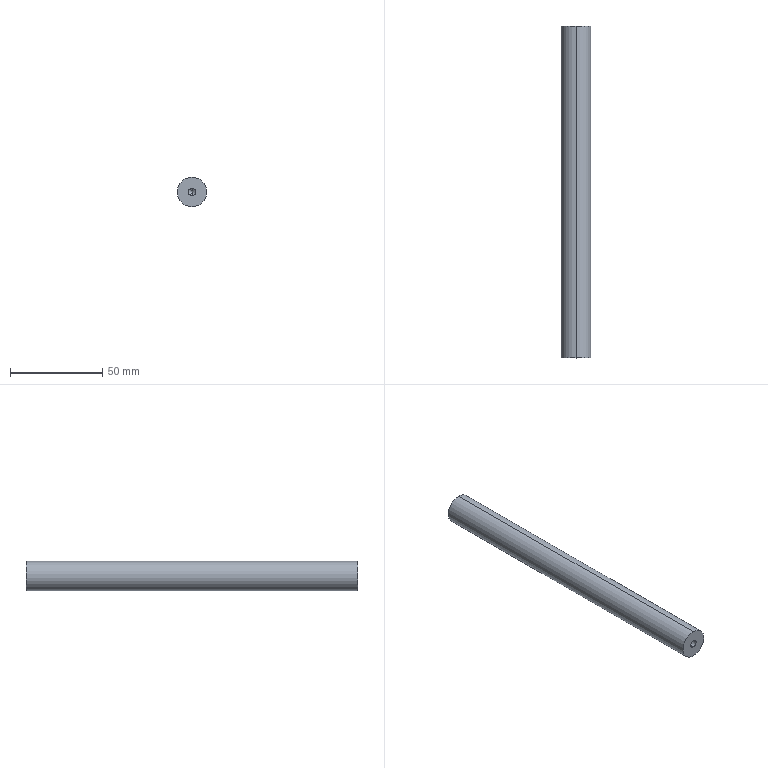Part | STEP file | PSFJW16-180-M5-N5 | 1 solid | 12 faces | box 16 x 180 x 16 mm | volume 35836 mm3 | cylinder 6 | cone 4 | plane 2 | commonest cylinder face diameters 4.2 x4 16 x2
STEP:
#1=CARTESIAN_POINT('',(0.,0.,0.));
#2=DIRECTION('',(0.,0.,1.));
#3=DIRECTION('',(1.,0.,0.));
#4=AXIS2_PLACEMENT_3D('',#1,#2,#3);
#5=CARTESIAN_POINT('',(0.,12.4,-2.1));
#6=VERTEX_POINT('',#5);
#7=CARTESIAN_POINT('',(0.,0.,-2.1));
#8=VERTEX_POINT('',#7);
#9=CARTESIAN_POINT('',(0.,0.,-2.1));
#10=DIRECTION('',(0.,-1.,0.));
#11=VECTOR('',#10,1.);
#12=LINE('',#9,#11);
#13=CARTESIAN_POINT('',(0.,0.,0.));
#14=DIRECTION('',(0.,-1.,0.));
#15=DIRECTION('',(0.,0.,-1.));
#16=AXIS2_PLACEMENT_3D('',#13,#14,#15);
#17=CYLINDRICAL_SURFACE('',#16,2.1);
#18=CARTESIAN_POINT('',(6.283,0.));
#19=DIRECTION('',(0.,1.));
#20=VECTOR('',#19,1.);
#21=LINE('',#18,#20);
#22=(GEOMETRIC_REPRESENTATION_CONTEXT(2)PARAMETRIC_REPRESENTATION_CONTEXT()REPRESENTATION_CONTEXT('',''));
#23=DEFINITIONAL_REPRESENTATION('',(#21),#22);
#24=PCURVE('',#17,#23);
#25=CARTESIAN_POINT('',(0.,0.,0.));
#26=DIRECTION('',(0.,-1.,0.));
#27=DIRECTION('',(0.,0.,-1.));
#28=AXIS2_PLACEMENT_3D('',#25,#26,#27);
#29=CYLINDRICAL_SURFACE('',#28,2.1);
#30=CARTESIAN_POINT('',(0.,0.));
#31=DIRECTION('',(0.,1.));
#32=VECTOR('',#31,1.);
#33=LINE('',#30,#32);
#34=(GEOMETRIC_REPRESENTATION_CONTEXT(2)PARAMETRIC_REPRESENTATION_CONTEXT()REPRESENTATION_CONTEXT('',''));
#35=DEFINITIONAL_REPRESENTATION('',(#33),#34);
#36=PCURVE('',#29,#35);
#37=SURFACE_CURVE('',#12,(#24,#36),.PCURVE_S1.);
#38=EDGE_CURVE('',#6,#8,#37,.T.);
#39=ORIENTED_EDGE('',*,*,#38,.T.);
#40=CARTESIAN_POINT('',(0.,0.,2.1));
#41=VERTEX_POINT('',#40);
#42=CARTESIAN_POINT('',(0.,0.,0.));
#43=DIRECTION('',(0.,-1.,0.));
#44=DIRECTION('',(0.,0.,-1.));
#45=AXIS2_PLACEMENT_3D('',#42,#43,#44);
#46=CIRCLE('',#45,2.1);
#47=CARTESIAN_POINT('',(0.,0.));
#48=DIRECTION('',(1.,0.));
#49=VECTOR('',#48,1.);
#50=LINE('',#47,#49);
#51=(GEOMETRIC_REPRESENTATION_CONTEXT(2)PARAMETRIC_REPRESENTATION_CONTEXT()REPRESENTATION_CONTEXT('',''));
#52=DEFINITIONAL_REPRESENTATION('',(#50),#51);
#53=PCURVE('',#17,#52);
#54=CARTESIAN_POINT('',(0.,0.,0.));
#55=DIRECTION('',(0.,1.,0.));
#56=DIRECTION('',(0.,0.,1.));
#57=AXIS2_PLACEMENT_3D('',#54,#55,#56);
#58=PLANE('',#57);
#59=CARTESIAN_POINT('',(-2.1,0.));
#60=CARTESIAN_POINT('',(-2.1,3.637));
#61=CARTESIAN_POINT('',(1.05,1.819));
#62=CARTESIAN_POINT('',(4.2,0.));
#63=CARTESIAN_POINT('',(1.05,-1.819));
#64=CARTESIAN_POINT('',(-2.1,-3.637));
#65=CARTESIAN_POINT('',(-2.1,0.));
#66=(BOUNDED_CURVE()B_SPLINE_CURVE(2,(#59,#60,#61,#62,#63,#64,#65),.UNSPECIFIED.,.T.,.F.)B_SPLINE_CURVE_WITH_KNOTS((1,2,2,2,2,1),(-2.094,0.,2.094,4.189,6.283,8.378),.UNSPECIFIED.)CURVE()GEOMETRIC_REPRESENTATION_ITEM()RATIONAL_B_SPLINE_CURVE((1.,0.5,1.,0.5,1.,0.5,1.))REPRESENTATION_ITEM(''));
#67=(GEOMETRIC_REPRESENTATION_CONTEXT(2)PARAMETRIC_REPRESENTATION_CONTEXT()REPRESENTATION_CONTEXT('',''));
#68=DEFINITIONAL_REPRESENTATION('',(#66),#67);
#69=PCURVE('',#58,#68);
#70=SURFACE_CURVE('',#46,(#53,#69),.PCURVE_S1.);
#71=EDGE_CURVE('',#41,#8,#70,.T.);
#72=ORIENTED_EDGE('',*,*,#71,.F.);
#73=CARTESIAN_POINT('',(0.,12.4,2.1));
#74=VERTEX_POINT('',#73);
#75=CARTESIAN_POINT('',(0.,0.,2.1));
#76=DIRECTION('',(0.,-1.,0.));
#77=VECTOR('',#76,1.);
#78=LINE('',#75,#77);
#79=CARTESIAN_POINT('',(3.142,0.));
#80=DIRECTION('',(0.,1.));
#81=VECTOR('',#80,1.);
#82=LINE('',#79,#81);
#83=(GEOMETRIC_REPRESENTATION_CONTEXT(2)PARAMETRIC_REPRESENTATION_CONTEXT()REPRESENTATION_CONTEXT('',''));
#84=DEFINITIONAL_REPRESENTATION('',(#82),#83);
#85=PCURVE('',#17,#84);
#86=CARTESIAN_POINT('',(3.142,0.));
#87=DIRECTION('',(0.,1.));
#88=VECTOR('',#87,1.);
#89=LINE('',#86,#88);
#90=(GEOMETRIC_REPRESENTATION_CONTEXT(2)PARAMETRIC_REPRESENTATION_CONTEXT()REPRESENTATION_CONTEXT('',''));
#91=DEFINITIONAL_REPRESENTATION('',(#89),#90);
#92=PCURVE('',#29,#91);
#93=SURFACE_CURVE('',#78,(#85,#92),.PCURVE_S1.);
#94=EDGE_CURVE('',#74,#41,#93,.T.);
#95=ORIENTED_EDGE('',*,*,#94,.F.);
#96=CARTESIAN_POINT('',(0.,12.4,0.));
#97=DIRECTION('',(0.,-1.,0.));
#98=DIRECTION('',(0.,0.,-1.));
#99=AXIS2_PLACEMENT_3D('',#96,#97,#98);
#100=CIRCLE('',#99,2.1);
#101=CARTESIAN_POINT('',(0.,-12.4));
#102=DIRECTION('',(1.,0.));
#103=VECTOR('',#102,1.);
#104=LINE('',#101,#103);
#105=(GEOMETRIC_REPRESENTATION_CONTEXT(2)PARAMETRIC_REPRESENTATION_CONTEXT()REPRESENTATION_CONTEXT('',''));
#106=DEFINITIONAL_REPRESENTATION('',(#104),#105);
#107=PCURVE('',#17,#106);
#108=CARTESIAN_POINT('',(0.,12.4,0.));
#109=DIRECTION('',(0.,-1.,0.));
#110=DIRECTION('',(0.,0.,-1.));
#111=AXIS2_PLACEMENT_3D('',#108,#109,#110);
#112=CONICAL_SURFACE('',#111,2.1,1.03);
#113=CARTESIAN_POINT('',(0.,0.));
#114=DIRECTION('',(1.,0.));
#115=VECTOR('',#114,1.);
#116=LINE('',#113,#115);
#117=(GEOMETRIC_REPRESENTATION_CONTEXT(2)PARAMETRIC_REPRESENTATION_CONTEXT()REPRESENTATION_CONTEXT('',''));
#118=DEFINITIONAL_REPRESENTATION('',(#116),#117);
#119=PCURVE('',#112,#118);
#120=SURFACE_CURVE('',#100,(#107,#119),.PCURVE_S1.);
#121=EDGE_CURVE('',#74,#6,#120,.T.);
#122=ORIENTED_EDGE('',*,*,#121,.T.);
#123=EDGE_LOOP('',(#39,#72,#95,#122));
#124=FACE_BOUND('',#123,.F.);
#125=ADVANCED_FACE('',(#124),#17,.F.);
#126=ORIENTED_EDGE('',*,*,#121,.F.);
#127=CARTESIAN_POINT('',(0.,13.662,0.));
#128=VERTEX_POINT('',#127);
#129=CARTESIAN_POINT('',(0.,12.4,2.1));
#130=DIRECTION('',(0.,-0.515,0.8572));
#131=VECTOR('',#130,1.);
#132=LINE('',#129,#131);
#133=CARTESIAN_POINT('',(3.142,0.));
#134=DIRECTION('',(0.,1.));
#135=VECTOR('',#134,1.);
#136=LINE('',#133,#135);
#137=(GEOMETRIC_REPRESENTATION_CONTEXT(2)PARAMETRIC_REPRESENTATION_CONTEXT()REPRESENTATION_CONTEXT('',''));
#138=DEFINITIONAL_REPRESENTATION('',(#136),#137);
#139=PCURVE('',#112,#138);
#140=CARTESIAN_POINT('',(0.,12.4,0.));
#141=DIRECTION('',(0.,-1.,0.));
#142=DIRECTION('',(0.,0.,-1.));
#143=AXIS2_PLACEMENT_3D('',#140,#141,#142);
#144=CONICAL_SURFACE('',#143,2.1,1.03);
#145=CARTESIAN_POINT('',(3.142,0.));
#146=DIRECTION('',(0.,1.));
#147=VECTOR('',#146,1.);
#148=LINE('',#145,#147);
#149=(GEOMETRIC_REPRESENTATION_CONTEXT(2)PARAMETRIC_REPRESENTATION_CONTEXT()REPRESENTATION_CONTEXT('',''));
#150=DEFINITIONAL_REPRESENTATION('',(#148),#149);
#151=PCURVE('',#144,#150);
#152=SURFACE_CURVE('',#132,(#139,#151),.PCURVE_S1.);
#153=EDGE_CURVE('',#128,#74,#152,.T.);
#154=ORIENTED_EDGE('',*,*,#153,.F.);
#155=CARTESIAN_POINT('',(0.,12.4,-2.1));
#156=DIRECTION('',(0.,-0.515,-0.8572));
#157=VECTOR('',#156,1.);
#158=LINE('',#155,#157);
#159=CARTESIAN_POINT('',(6.283,0.));
#160=DIRECTION('',(0.,1.));
#161=VECTOR('',#160,1.);
#162=LINE('',#159,#161);
#163=(GEOMETRIC_REPRESENTATION_CONTEXT(2)PARAMETRIC_REPRESENTATION_CONTEXT()REPRESENTATION_CONTEXT('',''));
#164=DEFINITIONAL_REPRESENTATION('',(#162),#163);
#165=PCURVE('',#112,#164);
#166=CARTESIAN_POINT('',(0.,0.));
#167=DIRECTION('',(0.,1.));
#168=VECTOR('',#167,1.);
#169=LINE('',#166,#168);
#170=(GEOMETRIC_REPRESENTATION_CONTEXT(2)PARAMETRIC_REPRESENTATION_CONTEXT()REPRESENTATION_CONTEXT('',''));
#171=DEFINITIONAL_REPRESENTATION('',(#169),#170);
#172=PCURVE('',#144,#171);
#173=SURFACE_CURVE('',#158,(#165,#172),.PCURVE_S1.);
#174=EDGE_CURVE('',#128,#6,#173,.T.);
#175=ORIENTED_EDGE('',*,*,#174,.T.);
#176=EDGE_LOOP('',(#126,#154,#175));
#177=FACE_BOUND('',#176,.F.);
#178=ADVANCED_FACE('',(#177),#112,.F.);
#179=CARTESIAN_POINT('',(0.,167.6,2.1));
#180=VERTEX_POINT('',#179);
#181=CARTESIAN_POINT('',(0.,180.,2.1));
#182=VERTEX_POINT('',#181);
#183=CARTESIAN_POINT('',(0.,180.,2.1));
#184=DIRECTION('',(0.,1.,0.));
#185=VECTOR('',#184,1.);
#186=LINE('',#183,#185);
#187=CARTESIAN_POINT('',(0.,180.,0.));
#188=DIRECTION('',(0.,1.,0.));
#189=DIRECTION('',(0.,0.,1.));
#190=AXIS2_PLACEMENT_3D('',#187,#188,#189);
#191=CYLINDRICAL_SURFACE('',#190,2.1);
#192=CARTESIAN_POINT('',(6.283,0.));
#193=DIRECTION('',(0.,1.));
#194=VECTOR('',#193,1.);
#195=LINE('',#192,#194);
#196=(GEOMETRIC_REPRESENTATION_CONTEXT(2)PARAMETRIC_REPRESENTATION_CONTEXT()REPRESENTATION_CONTEXT('',''));
#197=DEFINITIONAL_REPRESENTATION('',(#195),#196);
#198=PCURVE('',#191,#197);
#199=CARTESIAN_POINT('',(0.,180.,0.));
#200=DIRECTION('',(0.,1.,0.));
#201=DIRECTION('',(0.,0.,1.));
#202=AXIS2_PLACEMENT_3D('',#199,#200,#201);
#203=CYLINDRICAL_SURFACE('',#202,2.1);
#204=CARTESIAN_POINT('',(0.,0.));
#205=DIRECTION('',(0.,1.));
#206=VECTOR('',#205,1.);
#207=LINE('',#204,#206);
#208=(GEOMETRIC_REPRESENTATION_CONTEXT(2)PARAMETRIC_REPRESENTATION_CONTEXT()REPRESENTATION_CONTEXT('',''));
#209=DEFINITIONAL_REPRESENTATION('',(#207),#208);
#210=PCURVE('',#203,#209);
#211=SURFACE_CURVE('',#186,(#198,#210),.PCURVE_S1.);
#212=EDGE_CURVE('',#180,#182,#211,.T.);
#213=ORIENTED_EDGE('',*,*,#212,.T.);
#214=CARTESIAN_POINT('',(0.,180.,-2.1));
#215=VERTEX_POINT('',#214);
#216=CARTESIAN_POINT('',(0.,180.,0.));
#217=DIRECTION('',(0.,1.,0.));
#218=DIRECTION('',(0.,0.,1.));
#219=AXIS2_PLACEMENT_3D('',#216,#217,#218);
#220=CIRCLE('',#219,2.1);
#221=CARTESIAN_POINT('',(0.,0.));
#222=DIRECTION('',(1.,0.));
#223=VECTOR('',#222,1.);
#224=LINE('',#221,#223);
#225=(GEOMETRIC_REPRESENTATION_CONTEXT(2)PARAMETRIC_REPRESENTATION_CONTEXT()REPRESENTATION_CONTEXT('',''));
#226=DEFINITIONAL_REPRESENTATION('',(#224),#225);
#227=PCURVE('',#191,#226);
#228=CARTESIAN_POINT('',(0.,180.,0.));
#229=DIRECTION('',(0.,1.,0.));
#230=DIRECTION('',(0.,0.,1.));
#231=AXIS2_PLACEMENT_3D('',#228,#229,#230);
#232=PLANE('',#231);
#233=CARTESIAN_POINT('',(0.,0.));
#234=DIRECTION('',(1.,0.));
#235=AXIS2_PLACEMENT_2D('',#233,#234);
#236=CIRCLE('',#235,2.1);
#237=(GEOMETRIC_REPRESENTATION_CONTEXT(2)PARAMETRIC_REPRESENTATION_CONTEXT()REPRESENTATION_CONTEXT('',''));
#238=DEFINITIONAL_REPRESENTATION('',(#236),#237);
#239=PCURVE('',#232,#238);
#240=SURFACE_CURVE('',#220,(#227,#239),.PCURVE_S1.);
#241=EDGE_CURVE('',#215,#182,#240,.T.);
#242=ORIENTED_EDGE('',*,*,#241,.F.);
#243=CARTESIAN_POINT('',(0.,167.6,-2.1));
#244=VERTEX_POINT('',#243);
#245=CARTESIAN_POINT('',(0.,180.,-2.1));
#246=DIRECTION('',(0.,1.,0.));
#247=VECTOR('',#246,1.);
#248=LINE('',#245,#247);
#249=CARTESIAN_POINT('',(3.142,0.));
#250=DIRECTION('',(0.,1.));
#251=VECTOR('',#250,1.);
#252=LINE('',#249,#251);
#253=(GEOMETRIC_REPRESENTATION_CONTEXT(2)PARAMETRIC_REPRESENTATION_CONTEXT()REPRESENTATION_CONTEXT('',''));
#254=DEFINITIONAL_REPRESENTATION('',(#252),#253);
#255=PCURVE('',#191,#254);
#256=CARTESIAN_POINT('',(3.142,0.));
#257=DIRECTION('',(0.,1.));
#258=VECTOR('',#257,1.);
#259=LINE('',#256,#258);
#260=(GEOMETRIC_REPRESENTATION_CONTEXT(2)PARAMETRIC_REPRESENTATION_CONTEXT()REPRESENTATION_CONTEXT('',''));
#261=DEFINITIONAL_REPRESENTATION('',(#259),#260);
#262=PCURVE('',#203,#261);
#263=SURFACE_CURVE('',#248,(#255,#262),.PCURVE_S1.);
#264=EDGE_CURVE('',#244,#215,#263,.T.);
#265=ORIENTED_EDGE('',*,*,#264,.F.);
#266=CARTESIAN_POINT('',(0.,167.6,0.));
#267=DIRECTION('',(0.,1.,0.));
#268=DIRECTION('',(0.,0.,1.));
#269=AXIS2_PLACEMENT_3D('',#266,#267,#268);
#270=CIRCLE('',#269,2.1);
#271=CARTESIAN_POINT('',(0.,-12.4));
#272=DIRECTION('',(1.,0.));
#273=VECTOR('',#272,1.);
#274=LINE('',#271,#273);
#275=(GEOMETRIC_REPRESENTATION_CONTEXT(2)PARAMETRIC_REPRESENTATION_CONTEXT()REPRESENTATION_CONTEXT('',''));
#276=DEFINITIONAL_REPRESENTATION('',(#274),#275);
#277=PCURVE('',#191,#276);
#278=CARTESIAN_POINT('',(0.,167.6,0.));
#279=DIRECTION('',(0.,1.,0.));
#280=DIRECTION('',(0.,0.,1.));
#281=AXIS2_PLACEMENT_3D('',#278,#279,#280);
#282=CONICAL_SURFACE('',#281,2.1,1.03);
#283=CARTESIAN_POINT('',(0.,0.));
#284=DIRECTION('',(1.,0.));
#285=VECTOR('',#284,1.);
#286=LINE('',#283,#285);
#287=(GEOMETRIC_REPRESENTATION_CONTEXT(2)PARAMETRIC_REPRESENTATION_CONTEXT()REPRESENTATION_CONTEXT('',''));
#288=DEFINITIONAL_REPRESENTATION('',(#286),#287);
#289=PCURVE('',#282,#288);
#290=SURFACE_CURVE('',#270,(#277,#289),.PCURVE_S1.);
#291=EDGE_CURVE('',#244,#180,#290,.T.);
#292=ORIENTED_EDGE('',*,*,#291,.T.);
#293=EDGE_LOOP('',(#213,#242,#265,#292));
#294=FACE_BOUND('',#293,.F.);
#295=ADVANCED_FACE('',(#294),#191,.F.);
#296=ORIENTED_EDGE('',*,*,#291,.F.);
#297=CARTESIAN_POINT('',(0.,166.338,0.));
#298=VERTEX_POINT('',#297);
#299=CARTESIAN_POINT('',(0.,167.6,-2.1));
#300=DIRECTION('',(0.,0.515,-0.8572));
#301=VECTOR('',#300,1.);
#302=LINE('',#299,#301);
#303=CARTESIAN_POINT('',(3.142,0.));
#304=DIRECTION('',(0.,1.));
#305=VECTOR('',#304,1.);
#306=LINE('',#303,#305);
#307=(GEOMETRIC_REPRESENTATION_CONTEXT(2)PARAMETRIC_REPRESENTATION_CONTEXT()REPRESENTATION_CONTEXT('',''));
#308=DEFINITIONAL_REPRESENTATION('',(#306),#307);
#309=PCURVE('',#282,#308);
#310=CARTESIAN_POINT('',(0.,167.6,0.));
#311=DIRECTION('',(0.,1.,0.));
#312=DIRECTION('',(0.,0.,1.));
#313=AXIS2_PLACEMENT_3D('',#310,#311,#312);
#314=CONICAL_SURFACE('',#313,2.1,1.03);
#315=CARTESIAN_POINT('',(3.142,0.));
#316=DIRECTION('',(0.,1.));
#317=VECTOR('',#316,1.);
#318=LINE('',#315,#317);
#319=(GEOMETRIC_REPRESENTATION_CONTEXT(2)PARAMETRIC_REPRESENTATION_CONTEXT()REPRESENTATION_CONTEXT('',''));
#320=DEFINITIONAL_REPRESENTATION('',(#318),#319);
#321=PCURVE('',#314,#320);
#322=SURFACE_CURVE('',#302,(#309,#321),.PCURVE_S1.);
#323=EDGE_CURVE('',#298,#244,#322,.T.);
#324=ORIENTED_EDGE('',*,*,#323,.F.);
#325=CARTESIAN_POINT('',(0.,167.6,2.1));
#326=DIRECTION('',(0.,0.515,0.8572));
#327=VECTOR('',#326,1.);
#328=LINE('',#325,#327);
#329=CARTESIAN_POINT('',(6.283,0.));
#330=DIRECTION('',(0.,1.));
#331=VECTOR('',#330,1.);
#332=LINE('',#329,#331);
#333=(GEOMETRIC_REPRESENTATION_CONTEXT(2)PARAMETRIC_REPRESENTATION_CONTEXT()REPRESENTATION_CONTEXT('',''));
#334=DEFINITIONAL_REPRESENTATION('',(#332),#333);
#335=PCURVE('',#282,#334);
#336=CARTESIAN_POINT('',(0.,0.));
#337=DIRECTION('',(0.,1.));
#338=VECTOR('',#337,1.);
#339=LINE('',#336,#338);
#340=(GEOMETRIC_REPRESENTATION_CONTEXT(2)PARAMETRIC_REPRESENTATION_CONTEXT()REPRESENTATION_CONTEXT('',''));
#341=DEFINITIONAL_REPRESENTATION('',(#339),#340);
#342=PCURVE('',#314,#341);
#343=SURFACE_CURVE('',#328,(#335,#342),.PCURVE_S1.);
#344=EDGE_CURVE('',#298,#180,#343,.T.);
#345=ORIENTED_EDGE('',*,*,#344,.T.);
#346=EDGE_LOOP('',(#296,#324,#345));
#347=FACE_BOUND('',#346,.F.);
#348=ADVANCED_FACE('',(#347),#282,.F.);
#349=CARTESIAN_POINT('',(0.,180.,8.));
#350=VERTEX_POINT('',#349);
#351=CARTESIAN_POINT('',(0.,180.,-8.));
#352=VERTEX_POINT('',#351);
#353=CARTESIAN_POINT('',(0.,180.,0.));
#354=DIRECTION('',(0.,1.,0.));
#355=DIRECTION('',(0.,0.,1.));
#356=AXIS2_PLACEMENT_3D('',#353,#354,#355);
#357=CIRCLE('',#356,8.);
#358=CARTESIAN_POINT('',(0.,180.,0.));
#359=DIRECTION('',(0.,-1.,0.));
#360=DIRECTION('',(0.,0.,-1.));
#361=AXIS2_PLACEMENT_3D('',#358,#359,#360);
#362=CYLINDRICAL_SURFACE('',#361,8.);
#363=CARTESIAN_POINT('',(3.142,0.));
#364=DIRECTION('',(-1.,0.));
#365=VECTOR('',#364,1.);
#366=LINE('',#363,#365);
#367=(GEOMETRIC_REPRESENTATION_CONTEXT(2)PARAMETRIC_REPRESENTATION_CONTEXT()REPRESENTATION_CONTEXT('',''));
#368=DEFINITIONAL_REPRESENTATION('',(#366),#367);
#369=PCURVE('',#362,#368);
#370=CARTESIAN_POINT('',(0.,0.));
#371=DIRECTION('',(1.,0.));
#372=AXIS2_PLACEMENT_2D('',#370,#371);
#373=CIRCLE('',#372,8.);
#374=(GEOMETRIC_REPRESENTATION_CONTEXT(2)PARAMETRIC_REPRESENTATION_CONTEXT()REPRESENTATION_CONTEXT('',''));
#375=DEFINITIONAL_REPRESENTATION('',(#373),#374);
#376=PCURVE('',#232,#375);
#377=SURFACE_CURVE('',#357,(#369,#376),.PCURVE_S1.);
#378=EDGE_CURVE('',#350,#352,#377,.T.);
#379=ORIENTED_EDGE('',*,*,#378,.F.);
#380=CARTESIAN_POINT('',(0.,0.,8.));
#381=VERTEX_POINT('',#380);
#382=CARTESIAN_POINT('',(0.,180.,8.));
#383=DIRECTION('',(0.,-1.,0.));
#384=VECTOR('',#383,1.);
#385=LINE('',#382,#384);
#386=CARTESIAN_POINT('',(3.142,0.));
#387=DIRECTION('',(0.,1.));
#388=VECTOR('',#387,1.);
#389=LINE('',#386,#388);
#390=(GEOMETRIC_REPRESENTATION_CONTEXT(2)PARAMETRIC_REPRESENTATION_CONTEXT()REPRESENTATION_CONTEXT('',''));
#391=DEFINITIONAL_REPRESENTATION('',(#389),#390);
#392=PCURVE('',#362,#391);
#393=CARTESIAN_POINT('',(0.,180.,0.));
#394=DIRECTION('',(0.,-1.,0.));
#395=DIRECTION('',(0.,0.,-1.));
#396=AXIS2_PLACEMENT_3D('',#393,#394,#395);
#397=CYLINDRICAL_SURFACE('',#396,8.);
#398=CARTESIAN_POINT('',(3.142,0.));
#399=DIRECTION('',(0.,1.));
#400=VECTOR('',#399,1.);
#401=LINE('',#398,#400);
#402=(GEOMETRIC_REPRESENTATION_CONTEXT(2)PARAMETRIC_REPRESENTATION_CONTEXT()REPRESENTATION_CONTEXT('',''));
#403=DEFINITIONAL_REPRESENTATION('',(#401),#402);
#404=PCURVE('',#397,#403);
#405=SURFACE_CURVE('',#385,(#392,#404),.PCURVE_S1.);
#406=EDGE_CURVE('',#350,#381,#405,.T.);
#407=ORIENTED_EDGE('',*,*,#406,.T.);
#408=CARTESIAN_POINT('',(0.,0.,-8.));
#409=VERTEX_POINT('',#408);
#410=CARTESIAN_POINT('',(0.,0.,0.));
#411=DIRECTION('',(0.,1.,0.));
#412=DIRECTION('',(0.,0.,1.));
#413=AXIS2_PLACEMENT_3D('',#410,#411,#412);
#414=CIRCLE('',#413,8.);
#415=CARTESIAN_POINT('',(3.142,180.));
#416=DIRECTION('',(-1.,0.));
#417=VECTOR('',#416,1.);
#418=LINE('',#415,#417);
#419=(GEOMETRIC_REPRESENTATION_CONTEXT(2)PARAMETRIC_REPRESENTATION_CONTEXT()REPRESENTATION_CONTEXT('',''));
#420=DEFINITIONAL_REPRESENTATION('',(#418),#419);
#421=PCURVE('',#362,#420);
#422=CARTESIAN_POINT('',(0.,0.));
#423=DIRECTION('',(1.,0.));
#424=AXIS2_PLACEMENT_2D('',#422,#423);
#425=CIRCLE('',#424,8.);
#426=(GEOMETRIC_REPRESENTATION_CONTEXT(2)PARAMETRIC_REPRESENTATION_CONTEXT()REPRESENTATION_CONTEXT('',''));
#427=DEFINITIONAL_REPRESENTATION('',(#425),#426);
#428=PCURVE('',#58,#427);
#429=SURFACE_CURVE('',#414,(#421,#428),.PCURVE_S1.);
#430=EDGE_CURVE('',#381,#409,#429,.T.);
#431=ORIENTED_EDGE('',*,*,#430,.T.);
#432=CARTESIAN_POINT('',(0.,180.,-8.));
#433=DIRECTION('',(0.,-1.,0.));
#434=VECTOR('',#433,1.);
#435=LINE('',#432,#434);
#436=CARTESIAN_POINT('',(0.,0.));
#437=DIRECTION('',(0.,1.));
#438=VECTOR('',#437,1.);
#439=LINE('',#436,#438);
#440=(GEOMETRIC_REPRESENTATION_CONTEXT(2)PARAMETRIC_REPRESENTATION_CONTEXT()REPRESENTATION_CONTEXT('',''));
#441=DEFINITIONAL_REPRESENTATION('',(#439),#440);
#442=PCURVE('',#362,#441);
#443=CARTESIAN_POINT('',(6.283,0.));
#444=DIRECTION('',(0.,1.));
#445=VECTOR('',#444,1.);
#446=LINE('',#443,#445);
#447=(GEOMETRIC_REPRESENTATION_CONTEXT(2)PARAMETRIC_REPRESENTATION_CONTEXT()REPRESENTATION_CONTEXT('',''));
#448=DEFINITIONAL_REPRESENTATION('',(#446),#447);
#449=PCURVE('',#397,#448);
#450=SURFACE_CURVE('',#435,(#442,#449),.PCURVE_S1.);
#451=EDGE_CURVE('',#352,#409,#450,.T.);
#452=ORIENTED_EDGE('',*,*,#451,.F.);
#453=EDGE_LOOP('',(#379,#407,#431,#452));
#454=FACE_BOUND('',#453,.T.);
#455=ADVANCED_FACE('',(#454),#362,.T.);
#456=ORIENTED_EDGE('',*,*,#406,.F.);
#457=CARTESIAN_POINT('',(0.,180.,0.));
#458=DIRECTION('',(0.,1.,0.));
#459=DIRECTION('',(0.,0.,1.));
#460=AXIS2_PLACEMENT_3D('',#457,#458,#459);
#461=CIRCLE('',#460,8.);
#462=CARTESIAN_POINT('',(9.425,0.));
#463=DIRECTION('',(-1.,0.));
#464=VECTOR('',#463,1.);
#465=LINE('',#462,#464);
#466=(GEOMETRIC_REPRESENTATION_CONTEXT(2)PARAMETRIC_REPRESENTATION_CONTEXT()REPRESENTATION_CONTEXT('',''));
#467=DEFINITIONAL_REPRESENTATION('',(#465),#466);
#468=PCURVE('',#397,#467);
#469=CARTESIAN_POINT('',(0.,0.));
#470=DIRECTION('',(1.,0.));
#471=AXIS2_PLACEMENT_2D('',#469,#470);
#472=CIRCLE('',#471,8.);
#473=(GEOMETRIC_REPRESENTATION_CONTEXT(2)PARAMETRIC_REPRESENTATION_CONTEXT()REPRESENTATION_CONTEXT('',''));
#474=DEFINITIONAL_REPRESENTATION('',(#472),#473);
#475=PCURVE('',#232,#474);
#476=SURFACE_CURVE('',#461,(#468,#475),.PCURVE_S1.);
#477=EDGE_CURVE('',#352,#350,#476,.T.);
#478=ORIENTED_EDGE('',*,*,#477,.F.);
#479=ORIENTED_EDGE('',*,*,#451,.T.);
#480=CARTESIAN_POINT('',(0.,0.,0.));
#481=DIRECTION('',(0.,1.,0.));
#482=DIRECTION('',(0.,0.,1.));
#483=AXIS2_PLACEMENT_3D('',#480,#481,#482);
#484=CIRCLE('',#483,8.);
#485=CARTESIAN_POINT('',(9.425,180.));
#486=DIRECTION('',(-1.,0.));
#487=VECTOR('',#486,1.);
#488=LINE('',#485,#487);
#489=(GEOMETRIC_REPRESENTATION_CONTEXT(2)PARAMETRIC_REPRESENTATION_CONTEXT()REPRESENTATION_CONTEXT('',''));
#490=DEFINITIONAL_REPRESENTATION('',(#488),#489);
#491=PCURVE('',#397,#490);
#492=CARTESIAN_POINT('',(0.,0.));
#493=DIRECTION('',(1.,0.));
#494=AXIS2_PLACEMENT_2D('',#492,#493);
#495=CIRCLE('',#494,8.);
#496=(GEOMETRIC_REPRESENTATION_CONTEXT(2)PARAMETRIC_REPRESENTATION_CONTEXT()REPRESENTATION_CONTEXT('',''));
#497=DEFINITIONAL_REPRESENTATION('',(#495),#496);
#498=PCURVE('',#58,#497);
#499=SURFACE_CURVE('',#484,(#491,#498),.PCURVE_S1.);
#500=EDGE_CURVE('',#409,#381,#499,.T.);
#501=ORIENTED_EDGE('',*,*,#500,.T.);
#502=EDGE_LOOP('',(#456,#478,#479,#501));
#503=FACE_BOUND('',#502,.T.);
#504=ADVANCED_FACE('',(#503),#397,.T.);
#505=CARTESIAN_POINT('',(0.,180.,0.));
#506=DIRECTION('',(0.,1.,0.));
#507=DIRECTION('',(0.,0.,1.));
#508=AXIS2_PLACEMENT_3D('',#505,#506,#507);
#509=CIRCLE('',#508,2.1);
#510=CARTESIAN_POINT('',(0.,0.));
#511=DIRECTION('',(1.,0.));
#512=AXIS2_PLACEMENT_2D('',#510,#511);
#513=CIRCLE('',#512,2.1);
#514=(GEOMETRIC_REPRESENTATION_CONTEXT(2)PARAMETRIC_REPRESENTATION_CONTEXT()REPRESENTATION_CONTEXT('',''));
#515=DEFINITIONAL_REPRESENTATION('',(#513),#514);
#516=PCURVE('',#232,#515);
#517=CARTESIAN_POINT('',(0.,0.));
#518=DIRECTION('',(1.,0.));
#519=VECTOR('',#518,1.);
#520=LINE('',#517,#519);
#521=(GEOMETRIC_REPRESENTATION_CONTEXT(2)PARAMETRIC_REPRESENTATION_CONTEXT()REPRESENTATION_CONTEXT('',''));
#522=DEFINITIONAL_REPRESENTATION('',(#520),#521);
#523=PCURVE('',#203,#522);
#524=SURFACE_CURVE('',#509,(#516,#523),.PCURVE_S1.);
#525=EDGE_CURVE('',#182,#215,#524,.T.);
#526=ORIENTED_EDGE('',*,*,#525,.F.);
#527=ORIENTED_EDGE('',*,*,#241,.F.);
#528=EDGE_LOOP('',(#526,#527));
#529=FACE_BOUND('',#528,.T.);
#530=ORIENTED_EDGE('',*,*,#477,.T.);
#531=ORIENTED_EDGE('',*,*,#378,.T.);
#532=EDGE_LOOP('',(#530,#531));
#533=FACE_BOUND('',#532,.T.);
#534=ADVANCED_FACE('',(#529,#533),#232,.T.);
#535=CARTESIAN_POINT('',(0.,0.,0.));
#536=DIRECTION('',(0.,-1.,0.));
#537=DIRECTION('',(0.,0.,-1.));
#538=AXIS2_PLACEMENT_3D('',#535,#536,#537);
#539=CIRCLE('',#538,2.1);
#540=CARTESIAN_POINT('',(-2.1,0.));
#541=CARTESIAN_POINT('',(-2.1,3.637));
#542=CARTESIAN_POINT('',(1.05,1.819));
#543=CARTESIAN_POINT('',(4.2,0.));
#544=CARTESIAN_POINT('',(1.05,-1.819));
#545=CARTESIAN_POINT('',(-2.1,-3.637));
#546=CARTESIAN_POINT('',(-2.1,0.));
#547=(BOUNDED_CURVE()B_SPLINE_CURVE(2,(#540,#541,#542,#543,#544,#545,#546),.UNSPECIFIED.,.T.,.F.)B_SPLINE_CURVE_WITH_KNOTS((1,2,2,2,2,1),(-2.094,0.,2.094,4.189,6.283,8.378),.UNSPECIFIED.)CURVE()GEOMETRIC_REPRESENTATION_ITEM()RATIONAL_B_SPLINE_CURVE((1.,0.5,1.,0.5,1.,0.5,1.))REPRESENTATION_ITEM(''));
#548=(GEOMETRIC_REPRESENTATION_CONTEXT(2)PARAMETRIC_REPRESENTATION_CONTEXT()REPRESENTATION_CONTEXT('',''));
#549=DEFINITIONAL_REPRESENTATION('',(#547),#548);
#550=PCURVE('',#58,#549);
#551=CARTESIAN_POINT('',(0.,0.));
#552=DIRECTION('',(1.,0.));
#553=VECTOR('',#552,1.);
#554=LINE('',#551,#553);
#555=(GEOMETRIC_REPRESENTATION_CONTEXT(2)PARAMETRIC_REPRESENTATION_CONTEXT()REPRESENTATION_CONTEXT('',''));
#556=DEFINITIONAL_REPRESENTATION('',(#554),#555);
#557=PCURVE('',#29,#556);
#558=SURFACE_CURVE('',#539,(#550,#557),.PCURVE_S1.);
#559=EDGE_CURVE('',#8,#41,#558,.T.);
#560=ORIENTED_EDGE('',*,*,#559,.F.);
#561=ORIENTED_EDGE('',*,*,#71,.F.);
#562=EDGE_LOOP('',(#560,#561));
#563=FACE_BOUND('',#562,.T.);
#564=ORIENTED_EDGE('',*,*,#500,.F.);
#565=ORIENTED_EDGE('',*,*,#430,.F.);
#566=EDGE_LOOP('',(#564,#565));
#567=FACE_BOUND('',#566,.T.);
#568=ADVANCED_FACE('',(#563,#567),#58,.F.);
#569=CARTESIAN_POINT('',(0.,167.6,0.));
#570=DIRECTION('',(0.,1.,0.));
#571=DIRECTION('',(0.,0.,1.));
#572=AXIS2_PLACEMENT_3D('',#569,#570,#571);
#573=CIRCLE('',#572,2.1);
#574=CARTESIAN_POINT('',(0.,0.));
#575=DIRECTION('',(1.,0.));
#576=VECTOR('',#575,1.);
#577=LINE('',#574,#576);
#578=(GEOMETRIC_REPRESENTATION_CONTEXT(2)PARAMETRIC_REPRESENTATION_CONTEXT()REPRESENTATION_CONTEXT('',''));
#579=DEFINITIONAL_REPRESENTATION('',(#577),#578);
#580=PCURVE('',#314,#579);
#581=CARTESIAN_POINT('',(0.,-12.4));
#582=DIRECTION('',(1.,0.));
#583=VECTOR('',#582,1.);
#584=LINE('',#581,#583);
#585=(GEOMETRIC_REPRESENTATION_CONTEXT(2)PARAMETRIC_REPRESENTATION_CONTEXT()REPRESENTATION_CONTEXT('',''));
#586=DEFINITIONAL_REPRESENTATION('',(#584),#585);
#587=PCURVE('',#203,#586);
#588=SURFACE_CURVE('',#573,(#580,#587),.PCURVE_S1.);
#589=EDGE_CURVE('',#180,#244,#588,.T.);
#590=ORIENTED_EDGE('',*,*,#589,.F.);
#591=ORIENTED_EDGE('',*,*,#344,.F.);
#592=ORIENTED_EDGE('',*,*,#323,.T.);
#593=EDGE_LOOP('',(#590,#591,#592));
#594=FACE_BOUND('',#593,.F.);
#595=ADVANCED_FACE('',(#594),#314,.F.);
#596=ORIENTED_EDGE('',*,*,#525,.F.);
#597=ORIENTED_EDGE('',*,*,#212,.F.);
#598=ORIENTED_EDGE('',*,*,#589,.T.);
#599=ORIENTED_EDGE('',*,*,#264,.T.);
#600=EDGE_LOOP('',(#596,#597,#598,#599));
#601=FACE_BOUND('',#600,.F.);
#602=ADVANCED_FACE('',(#601),#203,.F.);
#603=CARTESIAN_POINT('',(0.,12.4,0.));
#604=DIRECTION('',(0.,-1.,0.));
#605=DIRECTION('',(0.,0.,-1.));
#606=AXIS2_PLACEMENT_3D('',#603,#604,#605);
#607=CIRCLE('',#606,2.1);
#608=CARTESIAN_POINT('',(0.,0.));
#609=DIRECTION('',(1.,0.));
#610=VECTOR('',#609,1.);
#611=LINE('',#608,#610);
#612=(GEOMETRIC_REPRESENTATION_CONTEXT(2)PARAMETRIC_REPRESENTATION_CONTEXT()REPRESENTATION_CONTEXT('',''));
#613=DEFINITIONAL_REPRESENTATION('',(#611),#612);
#614=PCURVE('',#144,#613);
#615=CARTESIAN_POINT('',(0.,-12.4));
#616=DIRECTION('',(1.,0.));
#617=VECTOR('',#616,1.);
#618=LINE('',#615,#617);
#619=(GEOMETRIC_REPRESENTATION_CONTEXT(2)PARAMETRIC_REPRESENTATION_CONTEXT()REPRESENTATION_CONTEXT('',''));
#620=DEFINITIONAL_REPRESENTATION('',(#618),#619);
#621=PCURVE('',#29,#620);
#622=SURFACE_CURVE('',#607,(#614,#621),.PCURVE_S1.);
#623=EDGE_CURVE('',#6,#74,#622,.T.);
#624=ORIENTED_EDGE('',*,*,#623,.F.);
#625=ORIENTED_EDGE('',*,*,#174,.F.);
#626=ORIENTED_EDGE('',*,*,#153,.T.);
#627=EDGE_LOOP('',(#624,#625,#626));
#628=FACE_BOUND('',#627,.F.);
#629=ADVANCED_FACE('',(#628),#144,.F.);
#630=ORIENTED_EDGE('',*,*,#559,.F.);
#631=ORIENTED_EDGE('',*,*,#38,.F.);
#632=ORIENTED_EDGE('',*,*,#623,.T.);
#633=ORIENTED_EDGE('',*,*,#94,.T.);
#634=EDGE_LOOP('',(#630,#631,#632,#633));
#635=FACE_BOUND('',#634,.F.);
#636=ADVANCED_FACE('',(#635),#29,.F.);
#637=CLOSED_SHELL('',(#125,#178,#295,#348,#455,#504,#534,#568,#595,#602,#629,#636));
#638=MANIFOLD_SOLID_BREP('',#637);
#639=(LENGTH_UNIT()NAMED_UNIT(*)SI_UNIT(.MILLI.,.METRE.));
#640=UNCERTAINTY_MEASURE_WITH_UNIT(LENGTH_MEASURE(0.0000001),#639,'','');
#641=(NAMED_UNIT(*)PLANE_ANGLE_UNIT()SI_UNIT($,.RADIAN.));
#642=(NAMED_UNIT(*)SI_UNIT($,.STERADIAN.)SOLID_ANGLE_UNIT());
#643=(GEOMETRIC_REPRESENTATION_CONTEXT(3)GLOBAL_UNCERTAINTY_ASSIGNED_CONTEXT((#640))GLOBAL_UNIT_ASSIGNED_CONTEXT((#639,#641,#642))REPRESENTATION_CONTEXT('',''));
#644=ADVANCED_BREP_SHAPE_REPRESENTATION('',(#4,#638),#643);